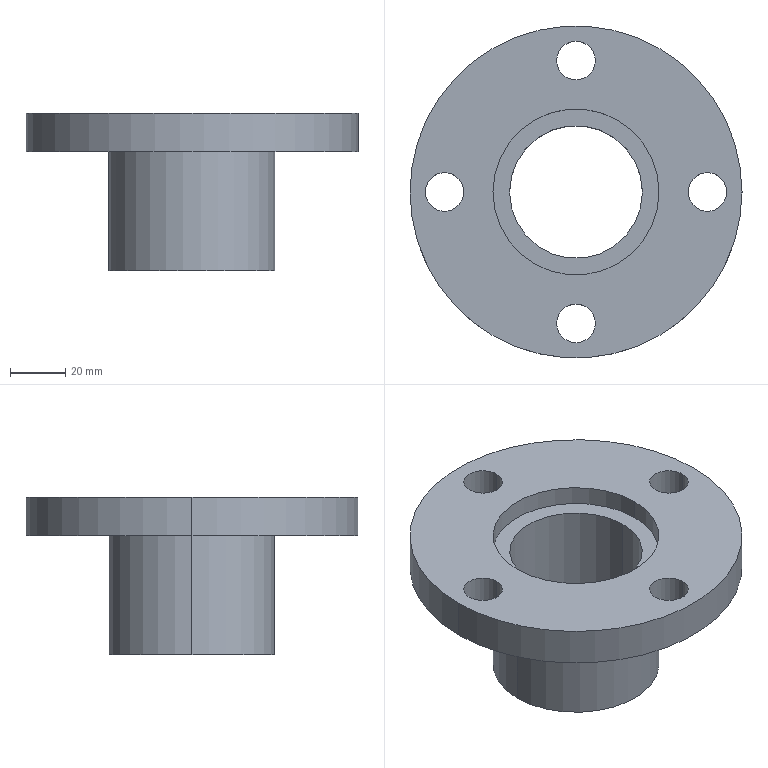Part | SolidWorks | features ExtruThin 1, HoleWzd 1, ICE 1 | 2 solids | 20 faces | box 120 x 120 x 57 mm | volume 161025 mm3 | cylinder 16 | plane 4 | commonest cylinder face diameters 14 x8 60 x4 48 x2 120 x2
STEP:
#1=CARTESIAN_POINT('',(-24.,0.,50.));
#2=VERTEX_POINT('',#1);
#3=CARTESIAN_POINT('',(24.,0.,50.));
#4=VERTEX_POINT('',#3);
#5=CARTESIAN_POINT('',(0.,0.,50.));
#6=DIRECTION('',(0.,0.,1.));
#7=DIRECTION('',(1.,0.,0.));
#8=AXIS2_PLACEMENT_3D('',#5,#6,#7);
#9=CIRCLE('',#8,24.);
#10=EDGE_CURVE('',#2,#4,#9,.T.);
#11=ORIENTED_EDGE('',*,*,#10,.T.);
#12=CARTESIAN_POINT('',(24.,0.,0.));
#13=VERTEX_POINT('',#12);
#14=CARTESIAN_POINT('',(24.,0.,50.));
#15=DIRECTION('',(0.,0.,-1.));
#16=VECTOR('',#15,1000.);
#17=LINE('',#14,#16);
#18=EDGE_CURVE('',#4,#13,#17,.T.);
#19=ORIENTED_EDGE('',*,*,#18,.T.);
#20=CARTESIAN_POINT('',(-24.,0.,0.));
#21=VERTEX_POINT('',#20);
#22=CARTESIAN_POINT('',(0.,0.,0.));
#23=DIRECTION('',(0.,0.,1.));
#24=DIRECTION('',(1.,0.,0.));
#25=AXIS2_PLACEMENT_3D('',#22,#23,#24);
#26=CIRCLE('',#25,24.);
#27=EDGE_CURVE('',#21,#13,#26,.T.);
#28=ORIENTED_EDGE('',*,*,#27,.F.);
#29=CARTESIAN_POINT('',(-24.,0.,50.));
#30=DIRECTION('',(0.,0.,-1.));
#31=VECTOR('',#30,1000.);
#32=LINE('',#29,#31);
#33=EDGE_CURVE('',#2,#21,#32,.T.);
#34=ORIENTED_EDGE('',*,*,#33,.F.);
#35=EDGE_LOOP('',(#11,#19,#28,#34));
#36=FACE_OUTER_BOUND('',#35,.T.);
#37=CARTESIAN_POINT('',(0.,0.,50.));
#38=DIRECTION('',(0.,0.,-1.));
#39=DIRECTION('',(-1.,0.,0.));
#40=AXIS2_PLACEMENT_3D('',#37,#38,#39);
#41=CYLINDRICAL_SURFACE('',#40,24.);
#42=ADVANCED_FACE('',(#36),#41,.F.);
#43=CARTESIAN_POINT('',(30.,0.,50.));
#44=VERTEX_POINT('',#43);
#45=CARTESIAN_POINT('',(-30.,0.,50.));
#46=VERTEX_POINT('',#45);
#47=CARTESIAN_POINT('',(0.,0.,50.));
#48=DIRECTION('',(0.,0.,1.));
#49=DIRECTION('',(1.,0.,0.));
#50=AXIS2_PLACEMENT_3D('',#47,#48,#49);
#51=CIRCLE('',#50,30.);
#52=EDGE_CURVE('',#44,#46,#51,.T.);
#53=ORIENTED_EDGE('',*,*,#52,.F.);
#54=CARTESIAN_POINT('',(30.,0.,0.));
#55=VERTEX_POINT('',#54);
#56=CARTESIAN_POINT('',(30.,0.,50.));
#57=DIRECTION('',(0.,0.,-1.));
#58=VECTOR('',#57,1000.);
#59=LINE('',#56,#58);
#60=EDGE_CURVE('',#44,#55,#59,.T.);
#61=ORIENTED_EDGE('',*,*,#60,.T.);
#62=CARTESIAN_POINT('',(-30.,0.,0.));
#63=VERTEX_POINT('',#62);
#64=CARTESIAN_POINT('',(0.,0.,0.));
#65=DIRECTION('',(0.,0.,1.));
#66=DIRECTION('',(1.,0.,0.));
#67=AXIS2_PLACEMENT_3D('',#64,#65,#66);
#68=CIRCLE('',#67,30.);
#69=EDGE_CURVE('',#55,#63,#68,.T.);
#70=ORIENTED_EDGE('',*,*,#69,.T.);
#71=CARTESIAN_POINT('',(-30.,0.,50.));
#72=DIRECTION('',(0.,0.,-1.));
#73=VECTOR('',#72,1000.);
#74=LINE('',#71,#73);
#75=EDGE_CURVE('',#46,#63,#74,.T.);
#76=ORIENTED_EDGE('',*,*,#75,.F.);
#77=EDGE_LOOP('',(#53,#61,#70,#76));
#78=FACE_OUTER_BOUND('',#77,.T.);
#79=CARTESIAN_POINT('',(0.,0.,50.));
#80=DIRECTION('',(0.,0.,-1.));
#81=DIRECTION('',(-1.,0.,0.));
#82=AXIS2_PLACEMENT_3D('',#79,#80,#81);
#83=CYLINDRICAL_SURFACE('',#82,30.);
#84=ADVANCED_FACE('',(#78),#83,.T.);
#85=CARTESIAN_POINT('',(0.,0.,50.));
#86=DIRECTION('',(0.,0.,1.));
#87=DIRECTION('',(1.,0.,0.));
#88=AXIS2_PLACEMENT_3D('',#85,#86,#87);
#89=CIRCLE('',#88,30.);
#90=EDGE_CURVE('',#46,#44,#89,.T.);
#91=ORIENTED_EDGE('',*,*,#90,.T.);
#92=ORIENTED_EDGE('',*,*,#52,.T.);
#93=EDGE_LOOP('',(#91,#92));
#94=FACE_OUTER_BOUND('',#93,.T.);
#95=ORIENTED_EDGE('',*,*,#10,.F.);
#96=CARTESIAN_POINT('',(0.,0.,50.));
#97=DIRECTION('',(0.,0.,1.));
#98=DIRECTION('',(1.,0.,0.));
#99=AXIS2_PLACEMENT_3D('',#96,#97,#98);
#100=CIRCLE('',#99,24.);
#101=EDGE_CURVE('',#4,#2,#100,.T.);
#102=ORIENTED_EDGE('',*,*,#101,.F.);
#103=EDGE_LOOP('',(#95,#102));
#104=FACE_BOUND('',#103,.T.);
#105=CARTESIAN_POINT('',(0.,0.,50.));
#106=DIRECTION('',(0.,0.,1.));
#107=DIRECTION('',(1.,0.,0.));
#108=AXIS2_PLACEMENT_3D('',#105,#106,#107);
#109=PLANE('',#108);
#110=ADVANCED_FACE('',(#94,#104),#109,.T.);
#111=CARTESIAN_POINT('',(0.,0.,0.));
#112=DIRECTION('',(0.,0.,1.));
#113=DIRECTION('',(1.,0.,0.));
#114=AXIS2_PLACEMENT_3D('',#111,#112,#113);
#115=CIRCLE('',#114,30.);
#116=EDGE_CURVE('',#63,#55,#115,.T.);
#117=ORIENTED_EDGE('',*,*,#116,.F.);
#118=ORIENTED_EDGE('',*,*,#69,.F.);
#119=EDGE_LOOP('',(#117,#118));
#120=FACE_OUTER_BOUND('',#119,.T.);
#121=ORIENTED_EDGE('',*,*,#27,.T.);
#122=CARTESIAN_POINT('',(0.,0.,0.));
#123=DIRECTION('',(0.,0.,1.));
#124=DIRECTION('',(1.,0.,0.));
#125=AXIS2_PLACEMENT_3D('',#122,#123,#124);
#126=CIRCLE('',#125,24.);
#127=EDGE_CURVE('',#13,#21,#126,.T.);
#128=ORIENTED_EDGE('',*,*,#127,.T.);
#129=EDGE_LOOP('',(#121,#128));
#130=FACE_BOUND('',#129,.T.);
#131=CARTESIAN_POINT('',(0.,0.,0.));
#132=DIRECTION('',(0.,0.,1.));
#133=DIRECTION('',(1.,0.,0.));
#134=AXIS2_PLACEMENT_3D('',#131,#132,#133);
#135=PLANE('',#134);
#136=ADVANCED_FACE('',(#120,#130),#135,.F.);
#137=ORIENTED_EDGE('',*,*,#60,.F.);
#138=ORIENTED_EDGE('',*,*,#90,.F.);
#139=ORIENTED_EDGE('',*,*,#75,.T.);
#140=ORIENTED_EDGE('',*,*,#116,.T.);
#141=EDGE_LOOP('',(#137,#138,#139,#140));
#142=FACE_OUTER_BOUND('',#141,.T.);
#143=CARTESIAN_POINT('',(0.,0.,50.));
#144=DIRECTION('',(0.,0.,-1.));
#145=DIRECTION('',(-1.,0.,0.));
#146=AXIS2_PLACEMENT_3D('',#143,#144,#145);
#147=CYLINDRICAL_SURFACE('',#146,30.);
#148=ADVANCED_FACE('',(#142),#147,.T.);
#149=ORIENTED_EDGE('',*,*,#18,.F.);
#150=ORIENTED_EDGE('',*,*,#101,.T.);
#151=ORIENTED_EDGE('',*,*,#33,.T.);
#152=ORIENTED_EDGE('',*,*,#127,.F.);
#153=EDGE_LOOP('',(#149,#150,#151,#152));
#154=FACE_OUTER_BOUND('',#153,.T.);
#155=CARTESIAN_POINT('',(0.,0.,50.));
#156=DIRECTION('',(0.,0.,-1.));
#157=DIRECTION('',(-1.,0.,0.));
#158=AXIS2_PLACEMENT_3D('',#155,#156,#157);
#159=CYLINDRICAL_SURFACE('',#158,24.);
#160=ADVANCED_FACE('',(#154),#159,.F.);
#161=CLOSED_SHELL('',(#42,#84,#110,#136,#148,#160));
#162=MANIFOLD_SOLID_BREP('',#161);
#163=CARTESIAN_POINT('',(-7.,47.5,43.));
#164=VERTEX_POINT('',#163);
#165=CARTESIAN_POINT('',(7.,47.5,43.));
#166=VERTEX_POINT('',#165);
#167=CARTESIAN_POINT('',(0.,47.5,43.));
#168=DIRECTION('',(0.,0.,1.));
#169=DIRECTION('',(1.,0.,0.));
#170=AXIS2_PLACEMENT_3D('',#167,#168,#169);
#171=CIRCLE('',#170,7.);
#172=EDGE_CURVE('',#164,#166,#171,.T.);
#173=ORIENTED_EDGE('',*,*,#172,.F.);
#174=CARTESIAN_POINT('',(-7.,47.5,57.));
#175=VERTEX_POINT('',#174);
#176=CARTESIAN_POINT('',(-7.,47.5,57.));
#177=DIRECTION('',(0.,0.,1.));
#178=VECTOR('',#177,1000.);
#179=LINE('',#176,#178);
#180=EDGE_CURVE('',#164,#175,#179,.T.);
#181=ORIENTED_EDGE('',*,*,#180,.T.);
#182=CARTESIAN_POINT('',(7.,47.5,57.));
#183=VERTEX_POINT('',#182);
#184=CARTESIAN_POINT('',(0.,47.5,57.));
#185=DIRECTION('',(0.,0.,1.));
#186=DIRECTION('',(1.,0.,0.));
#187=AXIS2_PLACEMENT_3D('',#184,#185,#186);
#188=CIRCLE('',#187,7.);
#189=EDGE_CURVE('',#175,#183,#188,.T.);
#190=ORIENTED_EDGE('',*,*,#189,.T.);
#191=CARTESIAN_POINT('',(7.,47.5,57.));
#192=DIRECTION('',(0.,0.,1.));
#193=VECTOR('',#192,1000.);
#194=LINE('',#191,#193);
#195=EDGE_CURVE('',#166,#183,#194,.T.);
#196=ORIENTED_EDGE('',*,*,#195,.F.);
#197=EDGE_LOOP('',(#173,#181,#190,#196));
#198=FACE_OUTER_BOUND('',#197,.T.);
#199=CARTESIAN_POINT('',(0.,47.5,57.));
#200=DIRECTION('',(0.,0.,1.));
#201=DIRECTION('',(1.,0.,0.));
#202=AXIS2_PLACEMENT_3D('',#199,#200,#201);
#203=CYLINDRICAL_SURFACE('',#202,7.);
#204=ADVANCED_FACE('',(#198),#203,.F.);
#205=CARTESIAN_POINT('',(-54.5,0.,43.));
#206=VERTEX_POINT('',#205);
#207=CARTESIAN_POINT('',(-40.5,0.,43.));
#208=VERTEX_POINT('',#207);
#209=CARTESIAN_POINT('',(-47.5,0.,43.));
#210=DIRECTION('',(0.,0.,1.));
#211=DIRECTION('',(1.,0.,0.));
#212=AXIS2_PLACEMENT_3D('',#209,#210,#211);
#213=CIRCLE('',#212,7.);
#214=EDGE_CURVE('',#206,#208,#213,.T.);
#215=ORIENTED_EDGE('',*,*,#214,.F.);
#216=CARTESIAN_POINT('',(-54.5,0.,57.));
#217=VERTEX_POINT('',#216);
#218=CARTESIAN_POINT('',(-54.5,0.,57.));
#219=DIRECTION('',(0.,0.,1.));
#220=VECTOR('',#219,1000.);
#221=LINE('',#218,#220);
#222=EDGE_CURVE('',#206,#217,#221,.T.);
#223=ORIENTED_EDGE('',*,*,#222,.T.);
#224=CARTESIAN_POINT('',(-40.5,0.,57.));
#225=VERTEX_POINT('',#224);
#226=CARTESIAN_POINT('',(-47.5,0.,57.));
#227=DIRECTION('',(0.,0.,1.));
#228=DIRECTION('',(1.,0.,0.));
#229=AXIS2_PLACEMENT_3D('',#226,#227,#228);
#230=CIRCLE('',#229,7.);
#231=EDGE_CURVE('',#217,#225,#230,.T.);
#232=ORIENTED_EDGE('',*,*,#231,.T.);
#233=CARTESIAN_POINT('',(-40.5,0.,57.));
#234=DIRECTION('',(0.,0.,1.));
#235=VECTOR('',#234,1000.);
#236=LINE('',#233,#235);
#237=EDGE_CURVE('',#208,#225,#236,.T.);
#238=ORIENTED_EDGE('',*,*,#237,.F.);
#239=EDGE_LOOP('',(#215,#223,#232,#238));
#240=FACE_OUTER_BOUND('',#239,.T.);
#241=CARTESIAN_POINT('',(-47.5,0.,57.));
#242=DIRECTION('',(0.,0.,1.));
#243=DIRECTION('',(1.,0.,0.));
#244=AXIS2_PLACEMENT_3D('',#241,#242,#243);
#245=CYLINDRICAL_SURFACE('',#244,7.);
#246=ADVANCED_FACE('',(#240),#245,.F.);
#247=CARTESIAN_POINT('',(40.5,0.,43.));
#248=VERTEX_POINT('',#247);
#249=CARTESIAN_POINT('',(54.5,0.,43.));
#250=VERTEX_POINT('',#249);
#251=CARTESIAN_POINT('',(47.5,0.,43.));
#252=DIRECTION('',(0.,0.,1.));
#253=DIRECTION('',(1.,0.,0.));
#254=AXIS2_PLACEMENT_3D('',#251,#252,#253);
#255=CIRCLE('',#254,7.);
#256=EDGE_CURVE('',#248,#250,#255,.T.);
#257=ORIENTED_EDGE('',*,*,#256,.F.);
#258=CARTESIAN_POINT('',(40.5,0.,57.));
#259=VERTEX_POINT('',#258);
#260=CARTESIAN_POINT('',(40.5,0.,57.));
#261=DIRECTION('',(0.,0.,1.));
#262=VECTOR('',#261,1000.);
#263=LINE('',#260,#262);
#264=EDGE_CURVE('',#248,#259,#263,.T.);
#265=ORIENTED_EDGE('',*,*,#264,.T.);
#266=CARTESIAN_POINT('',(54.5,0.,57.));
#267=VERTEX_POINT('',#266);
#268=CARTESIAN_POINT('',(47.5,0.,57.));
#269=DIRECTION('',(0.,0.,1.));
#270=DIRECTION('',(1.,0.,0.));
#271=AXIS2_PLACEMENT_3D('',#268,#269,#270);
#272=CIRCLE('',#271,7.);
#273=EDGE_CURVE('',#259,#267,#272,.T.);
#274=ORIENTED_EDGE('',*,*,#273,.T.);
#275=CARTESIAN_POINT('',(54.5,0.,57.));
#276=DIRECTION('',(0.,0.,1.));
#277=VECTOR('',#276,1000.);
#278=LINE('',#275,#277);
#279=EDGE_CURVE('',#250,#267,#278,.T.);
#280=ORIENTED_EDGE('',*,*,#279,.F.);
#281=EDGE_LOOP('',(#257,#265,#274,#280));
#282=FACE_OUTER_BOUND('',#281,.T.);
#283=CARTESIAN_POINT('',(47.5,0.,57.));
#284=DIRECTION('',(0.,0.,1.));
#285=DIRECTION('',(1.,0.,0.));
#286=AXIS2_PLACEMENT_3D('',#283,#284,#285);
#287=CYLINDRICAL_SURFACE('',#286,7.);
#288=ADVANCED_FACE('',(#282),#287,.F.);
#289=CARTESIAN_POINT('',(-7.,-47.5,43.));
#290=VERTEX_POINT('',#289);
#291=CARTESIAN_POINT('',(7.,-47.5,43.));
#292=VERTEX_POINT('',#291);
#293=CARTESIAN_POINT('',(0.,-47.5,43.));
#294=DIRECTION('',(0.,0.,1.));
#295=DIRECTION('',(1.,0.,0.));
#296=AXIS2_PLACEMENT_3D('',#293,#294,#295);
#297=CIRCLE('',#296,7.);
#298=EDGE_CURVE('',#290,#292,#297,.T.);
#299=ORIENTED_EDGE('',*,*,#298,.F.);
#300=CARTESIAN_POINT('',(-7.,-47.5,57.));
#301=VERTEX_POINT('',#300);
#302=CARTESIAN_POINT('',(-7.,-47.5,57.));
#303=DIRECTION('',(0.,0.,1.));
#304=VECTOR('',#303,1000.);
#305=LINE('',#302,#304);
#306=EDGE_CURVE('',#290,#301,#305,.T.);
#307=ORIENTED_EDGE('',*,*,#306,.T.);
#308=CARTESIAN_POINT('',(7.,-47.5,57.));
#309=VERTEX_POINT('',#308);
#310=CARTESIAN_POINT('',(0.,-47.5,57.));
#311=DIRECTION('',(0.,0.,1.));
#312=DIRECTION('',(1.,0.,0.));
#313=AXIS2_PLACEMENT_3D('',#310,#311,#312);
#314=CIRCLE('',#313,7.);
#315=EDGE_CURVE('',#301,#309,#314,.T.);
#316=ORIENTED_EDGE('',*,*,#315,.T.);
#317=CARTESIAN_POINT('',(7.,-47.5,57.));
#318=DIRECTION('',(0.,0.,1.));
#319=VECTOR('',#318,1000.);
#320=LINE('',#317,#319);
#321=EDGE_CURVE('',#292,#309,#320,.T.);
#322=ORIENTED_EDGE('',*,*,#321,.F.);
#323=EDGE_LOOP('',(#299,#307,#316,#322));
#324=FACE_OUTER_BOUND('',#323,.T.);
#325=CARTESIAN_POINT('',(0.,-47.5,57.));
#326=DIRECTION('',(0.,0.,1.));
#327=DIRECTION('',(1.,0.,0.));
#328=AXIS2_PLACEMENT_3D('',#325,#326,#327);
#329=CYLINDRICAL_SURFACE('',#328,7.);
#330=ADVANCED_FACE('',(#324),#329,.F.);
#331=CARTESIAN_POINT('',(-30.,0.,57.));
#332=VERTEX_POINT('',#331);
#333=CARTESIAN_POINT('',(30.,0.,57.));
#334=VERTEX_POINT('',#333);
#335=CARTESIAN_POINT('',(0.,0.,57.));
#336=DIRECTION('',(0.,0.,1.));
#337=DIRECTION('',(1.,0.,0.));
#338=AXIS2_PLACEMENT_3D('',#335,#336,#337);
#339=CIRCLE('',#338,30.);
#340=EDGE_CURVE('',#332,#334,#339,.T.);
#341=ORIENTED_EDGE('',*,*,#340,.T.);
#342=CARTESIAN_POINT('',(30.,0.,43.));
#343=VERTEX_POINT('',#342);
#344=CARTESIAN_POINT('',(30.,0.,57.));
#345=DIRECTION('',(0.,0.,-1.));
#346=VECTOR('',#345,1000.);
#347=LINE('',#344,#346);
#348=EDGE_CURVE('',#334,#343,#347,.T.);
#349=ORIENTED_EDGE('',*,*,#348,.T.);
#350=CARTESIAN_POINT('',(-30.,0.,43.));
#351=VERTEX_POINT('',#350);
#352=CARTESIAN_POINT('',(0.,0.,43.));
#353=DIRECTION('',(0.,0.,1.));
#354=DIRECTION('',(1.,0.,0.));
#355=AXIS2_PLACEMENT_3D('',#352,#353,#354);
#356=CIRCLE('',#355,30.);
#357=EDGE_CURVE('',#351,#343,#356,.T.);
#358=ORIENTED_EDGE('',*,*,#357,.F.);
#359=CARTESIAN_POINT('',(-30.,0.,57.));
#360=DIRECTION('',(0.,0.,-1.));
#361=VECTOR('',#360,1000.);
#362=LINE('',#359,#361);
#363=EDGE_CURVE('',#332,#351,#362,.T.);
#364=ORIENTED_EDGE('',*,*,#363,.F.);
#365=EDGE_LOOP('',(#341,#349,#358,#364));
#366=FACE_OUTER_BOUND('',#365,.T.);
#367=CARTESIAN_POINT('',(0.,0.,57.));
#368=DIRECTION('',(0.,0.,-1.));
#369=DIRECTION('',(-1.,0.,0.));
#370=AXIS2_PLACEMENT_3D('',#367,#368,#369);
#371=CYLINDRICAL_SURFACE('',#370,30.);
#372=ADVANCED_FACE('',(#366),#371,.F.);
#373=CARTESIAN_POINT('',(60.,0.,57.));
#374=VERTEX_POINT('',#373);
#375=CARTESIAN_POINT('',(-60.,0.,57.));
#376=VERTEX_POINT('',#375);
#377=CARTESIAN_POINT('',(0.,0.,57.));
#378=DIRECTION('',(0.,0.,1.));
#379=DIRECTION('',(1.,0.,0.));
#380=AXIS2_PLACEMENT_3D('',#377,#378,#379);
#381=CIRCLE('',#380,60.);
#382=EDGE_CURVE('',#374,#376,#381,.T.);
#383=ORIENTED_EDGE('',*,*,#382,.F.);
#384=CARTESIAN_POINT('',(60.,0.,43.));
#385=VERTEX_POINT('',#384);
#386=CARTESIAN_POINT('',(60.,0.,57.));
#387=DIRECTION('',(0.,0.,-1.));
#388=VECTOR('',#387,1000.);
#389=LINE('',#386,#388);
#390=EDGE_CURVE('',#374,#385,#389,.T.);
#391=ORIENTED_EDGE('',*,*,#390,.T.);
#392=CARTESIAN_POINT('',(-60.,0.,43.));
#393=VERTEX_POINT('',#392);
#394=CARTESIAN_POINT('',(0.,0.,43.));
#395=DIRECTION('',(0.,0.,1.));
#396=DIRECTION('',(1.,0.,0.));
#397=AXIS2_PLACEMENT_3D('',#394,#395,#396);
#398=CIRCLE('',#397,60.);
#399=EDGE_CURVE('',#385,#393,#398,.T.);
#400=ORIENTED_EDGE('',*,*,#399,.T.);
#401=CARTESIAN_POINT('',(-60.,0.,57.));
#402=DIRECTION('',(0.,0.,-1.));
#403=VECTOR('',#402,1000.);
#404=LINE('',#401,#403);
#405=EDGE_CURVE('',#376,#393,#404,.T.);
#406=ORIENTED_EDGE('',*,*,#405,.F.);
#407=EDGE_LOOP('',(#383,#391,#400,#406));
#408=FACE_OUTER_BOUND('',#407,.T.);
#409=CARTESIAN_POINT('',(0.,0.,57.));
#410=DIRECTION('',(0.,0.,-1.));
#411=DIRECTION('',(-1.,0.,0.));
#412=AXIS2_PLACEMENT_3D('',#409,#410,#411);
#413=CYLINDRICAL_SURFACE('',#412,60.);
#414=ADVANCED_FACE('',(#408),#413,.T.);
#415=CARTESIAN_POINT('',(0.,47.5,57.));
#416=DIRECTION('',(0.,0.,1.));
#417=DIRECTION('',(1.,0.,0.));
#418=AXIS2_PLACEMENT_3D('',#415,#416,#417);
#419=CIRCLE('',#418,7.);
#420=EDGE_CURVE('',#183,#175,#419,.T.);
#421=ORIENTED_EDGE('',*,*,#420,.F.);
#422=ORIENTED_EDGE('',*,*,#189,.F.);
#423=EDGE_LOOP('',(#421,#422));
#424=FACE_BOUND('',#423,.T.);
#425=CARTESIAN_POINT('',(-47.5,0.,57.));
#426=DIRECTION('',(0.,0.,1.));
#427=DIRECTION('',(1.,0.,0.));
#428=AXIS2_PLACEMENT_3D('',#425,#426,#427);
#429=CIRCLE('',#428,7.);
#430=EDGE_CURVE('',#225,#217,#429,.T.);
#431=ORIENTED_EDGE('',*,*,#430,.F.);
#432=ORIENTED_EDGE('',*,*,#231,.F.);
#433=EDGE_LOOP('',(#431,#432));
#434=FACE_BOUND('',#433,.T.);
#435=CARTESIAN_POINT('',(47.5,0.,57.));
#436=DIRECTION('',(0.,0.,1.));
#437=DIRECTION('',(1.,0.,0.));
#438=AXIS2_PLACEMENT_3D('',#435,#436,#437);
#439=CIRCLE('',#438,7.);
#440=EDGE_CURVE('',#267,#259,#439,.T.);
#441=ORIENTED_EDGE('',*,*,#440,.F.);
#442=ORIENTED_EDGE('',*,*,#273,.F.);
#443=EDGE_LOOP('',(#441,#442));
#444=FACE_BOUND('',#443,.T.);
#445=CARTESIAN_POINT('',(0.,-47.5,57.));
#446=DIRECTION('',(0.,0.,1.));
#447=DIRECTION('',(1.,0.,0.));
#448=AXIS2_PLACEMENT_3D('',#445,#446,#447);
#449=CIRCLE('',#448,7.);
#450=EDGE_CURVE('',#309,#301,#449,.T.);
#451=ORIENTED_EDGE('',*,*,#450,.F.);
#452=ORIENTED_EDGE('',*,*,#315,.F.);
#453=EDGE_LOOP('',(#451,#452));
#454=FACE_BOUND('',#453,.T.);
#455=CARTESIAN_POINT('',(0.,0.,57.));
#456=DIRECTION('',(0.,0.,1.));
#457=DIRECTION('',(1.,0.,0.));
#458=AXIS2_PLACEMENT_3D('',#455,#456,#457);
#459=CIRCLE('',#458,60.);
#460=EDGE_CURVE('',#376,#374,#459,.T.);
#461=ORIENTED_EDGE('',*,*,#460,.T.);
#462=ORIENTED_EDGE('',*,*,#382,.T.);
#463=EDGE_LOOP('',(#461,#462));
#464=FACE_OUTER_BOUND('',#463,.T.);
#465=ORIENTED_EDGE('',*,*,#340,.F.);
#466=CARTESIAN_POINT('',(0.,0.,57.));
#467=DIRECTION('',(0.,0.,1.));
#468=DIRECTION('',(1.,0.,0.));
#469=AXIS2_PLACEMENT_3D('',#466,#467,#468);
#470=CIRCLE('',#469,30.);
#471=EDGE_CURVE('',#334,#332,#470,.T.);
#472=ORIENTED_EDGE('',*,*,#471,.F.);
#473=EDGE_LOOP('',(#465,#472));
#474=FACE_BOUND('',#473,.T.);
#475=CARTESIAN_POINT('',(0.,0.,57.));
#476=DIRECTION('',(0.,0.,1.));
#477=DIRECTION('',(1.,0.,0.));
#478=AXIS2_PLACEMENT_3D('',#475,#476,#477);
#479=PLANE('',#478);
#480=ADVANCED_FACE('',(#424,#434,#444,#454,#464,#474),#479,.T.);
#481=CARTESIAN_POINT('',(0.,47.5,43.));
#482=DIRECTION('',(0.,0.,1.));
#483=DIRECTION('',(1.,0.,0.));
#484=AXIS2_PLACEMENT_3D('',#481,#482,#483);
#485=CIRCLE('',#484,7.);
#486=EDGE_CURVE('',#166,#164,#485,.T.);
#487=ORIENTED_EDGE('',*,*,#486,.T.);
#488=ORIENTED_EDGE('',*,*,#172,.T.);
#489=EDGE_LOOP('',(#487,#488));
#490=FACE_BOUND('',#489,.T.);
#491=CARTESIAN_POINT('',(-47.5,0.,43.));
#492=DIRECTION('',(0.,0.,1.));
#493=DIRECTION('',(1.,0.,0.));
#494=AXIS2_PLACEMENT_3D('',#491,#492,#493);
#495=CIRCLE('',#494,7.);
#496=EDGE_CURVE('',#208,#206,#495,.T.);
#497=ORIENTED_EDGE('',*,*,#496,.T.);
#498=ORIENTED_EDGE('',*,*,#214,.T.);
#499=EDGE_LOOP('',(#497,#498));
#500=FACE_BOUND('',#499,.T.);
#501=CARTESIAN_POINT('',(47.5,0.,43.));
#502=DIRECTION('',(0.,0.,1.));
#503=DIRECTION('',(1.,0.,0.));
#504=AXIS2_PLACEMENT_3D('',#501,#502,#503);
#505=CIRCLE('',#504,7.);
#506=EDGE_CURVE('',#250,#248,#505,.T.);
#507=ORIENTED_EDGE('',*,*,#506,.T.);
#508=ORIENTED_EDGE('',*,*,#256,.T.);
#509=EDGE_LOOP('',(#507,#508));
#510=FACE_BOUND('',#509,.T.);
#511=CARTESIAN_POINT('',(0.,-47.5,43.));
#512=DIRECTION('',(0.,0.,1.));
#513=DIRECTION('',(1.,0.,0.));
#514=AXIS2_PLACEMENT_3D('',#511,#512,#513);
#515=CIRCLE('',#514,7.);
#516=EDGE_CURVE('',#292,#290,#515,.T.);
#517=ORIENTED_EDGE('',*,*,#516,.T.);
#518=ORIENTED_EDGE('',*,*,#298,.T.);
#519=EDGE_LOOP('',(#517,#518));
#520=FACE_BOUND('',#519,.T.);
#521=CARTESIAN_POINT('',(0.,0.,43.));
#522=DIRECTION('',(0.,0.,1.));
#523=DIRECTION('',(1.,0.,0.));
#524=AXIS2_PLACEMENT_3D('',#521,#522,#523);
#525=CIRCLE('',#524,60.);
#526=EDGE_CURVE('',#393,#385,#525,.T.);
#527=ORIENTED_EDGE('',*,*,#526,.F.);
#528=ORIENTED_EDGE('',*,*,#399,.F.);
#529=EDGE_LOOP('',(#527,#528));
#530=FACE_OUTER_BOUND('',#529,.T.);
#531=ORIENTED_EDGE('',*,*,#357,.T.);
#532=CARTESIAN_POINT('',(0.,0.,43.));
#533=DIRECTION('',(0.,0.,1.));
#534=DIRECTION('',(1.,0.,0.));
#535=AXIS2_PLACEMENT_3D('',#532,#533,#534);
#536=CIRCLE('',#535,30.);
#537=EDGE_CURVE('',#343,#351,#536,.T.);
#538=ORIENTED_EDGE('',*,*,#537,.T.);
#539=EDGE_LOOP('',(#531,#538));
#540=FACE_BOUND('',#539,.T.);
#541=CARTESIAN_POINT('',(0.,0.,43.));
#542=DIRECTION('',(0.,0.,1.));
#543=DIRECTION('',(1.,0.,0.));
#544=AXIS2_PLACEMENT_3D('',#541,#542,#543);
#545=PLANE('',#544);
#546=ADVANCED_FACE('',(#490,#500,#510,#520,#530,#540),#545,.F.);
#547=ORIENTED_EDGE('',*,*,#390,.F.);
#548=ORIENTED_EDGE('',*,*,#460,.F.);
#549=ORIENTED_EDGE('',*,*,#405,.T.);
#550=ORIENTED_EDGE('',*,*,#526,.T.);
#551=EDGE_LOOP('',(#547,#548,#549,#550));
#552=FACE_OUTER_BOUND('',#551,.T.);
#553=CARTESIAN_POINT('',(0.,0.,57.));
#554=DIRECTION('',(0.,0.,-1.));
#555=DIRECTION('',(-1.,0.,0.));
#556=AXIS2_PLACEMENT_3D('',#553,#554,#555);
#557=CYLINDRICAL_SURFACE('',#556,60.);
#558=ADVANCED_FACE('',(#552),#557,.T.);
#559=ORIENTED_EDGE('',*,*,#348,.F.);
#560=ORIENTED_EDGE('',*,*,#471,.T.);
#561=ORIENTED_EDGE('',*,*,#363,.T.);
#562=ORIENTED_EDGE('',*,*,#537,.F.);
#563=EDGE_LOOP('',(#559,#560,#561,#562));
#564=FACE_OUTER_BOUND('',#563,.T.);
#565=CARTESIAN_POINT('',(0.,0.,57.));
#566=DIRECTION('',(0.,0.,-1.));
#567=DIRECTION('',(-1.,0.,0.));
#568=AXIS2_PLACEMENT_3D('',#565,#566,#567);
#569=CYLINDRICAL_SURFACE('',#568,30.);
#570=ADVANCED_FACE('',(#564),#569,.F.);
#571=ORIENTED_EDGE('',*,*,#306,.F.);
#572=ORIENTED_EDGE('',*,*,#516,.F.);
#573=ORIENTED_EDGE('',*,*,#321,.T.);
#574=ORIENTED_EDGE('',*,*,#450,.T.);
#575=EDGE_LOOP('',(#571,#572,#573,#574));
#576=FACE_OUTER_BOUND('',#575,.T.);
#577=CARTESIAN_POINT('',(0.,-47.5,57.));
#578=DIRECTION('',(0.,0.,1.));
#579=DIRECTION('',(1.,0.,0.));
#580=AXIS2_PLACEMENT_3D('',#577,#578,#579);
#581=CYLINDRICAL_SURFACE('',#580,7.);
#582=ADVANCED_FACE('',(#576),#581,.F.);
#583=ORIENTED_EDGE('',*,*,#264,.F.);
#584=ORIENTED_EDGE('',*,*,#506,.F.);
#585=ORIENTED_EDGE('',*,*,#279,.T.);
#586=ORIENTED_EDGE('',*,*,#440,.T.);
#587=EDGE_LOOP('',(#583,#584,#585,#586));
#588=FACE_OUTER_BOUND('',#587,.T.);
#589=CARTESIAN_POINT('',(47.5,0.,57.));
#590=DIRECTION('',(0.,0.,1.));
#591=DIRECTION('',(1.,0.,0.));
#592=AXIS2_PLACEMENT_3D('',#589,#590,#591);
#593=CYLINDRICAL_SURFACE('',#592,7.);
#594=ADVANCED_FACE('',(#588),#593,.F.);
#595=ORIENTED_EDGE('',*,*,#222,.F.);
#596=ORIENTED_EDGE('',*,*,#496,.F.);
#597=ORIENTED_EDGE('',*,*,#237,.T.);
#598=ORIENTED_EDGE('',*,*,#430,.T.);
#599=EDGE_LOOP('',(#595,#596,#597,#598));
#600=FACE_OUTER_BOUND('',#599,.T.);
#601=CARTESIAN_POINT('',(-47.5,0.,57.));
#602=DIRECTION('',(0.,0.,1.));
#603=DIRECTION('',(1.,0.,0.));
#604=AXIS2_PLACEMENT_3D('',#601,#602,#603);
#605=CYLINDRICAL_SURFACE('',#604,7.);
#606=ADVANCED_FACE('',(#600),#605,.F.);
#607=ORIENTED_EDGE('',*,*,#180,.F.);
#608=ORIENTED_EDGE('',*,*,#486,.F.);
#609=ORIENTED_EDGE('',*,*,#195,.T.);
#610=ORIENTED_EDGE('',*,*,#420,.T.);
#611=EDGE_LOOP('',(#607,#608,#609,#610));
#612=FACE_OUTER_BOUND('',#611,.T.);
#613=CARTESIAN_POINT('',(0.,47.5,57.));
#614=DIRECTION('',(0.,0.,1.));
#615=DIRECTION('',(1.,0.,0.));
#616=AXIS2_PLACEMENT_3D('',#613,#614,#615);
#617=CYLINDRICAL_SURFACE('',#616,7.);
#618=ADVANCED_FACE('',(#612),#617,.F.);
#619=CLOSED_SHELL('',(#204,#246,#288,#330,#372,#414,#480,#546,#558,#570,#582,#594,#606,#618));
#620=MANIFOLD_SOLID_BREP('',#619);
#621=CARTESIAN_POINT('',(0.,0.,0.));
#622=DIRECTION('',(0.,0.,1.));
#623=DIRECTION('',(1.,0.,0.));
#624=AXIS2_PLACEMENT_3D('',#621,#622,#623);
#625=(LENGTH_UNIT()NAMED_UNIT(*)SI_UNIT(.MILLI.,.METRE.));
#626=UNCERTAINTY_MEASURE_WITH_UNIT(LENGTH_MEASURE(0.00001),#625,'','');
#627=(NAMED_UNIT(*)PLANE_ANGLE_UNIT()SI_UNIT($,.RADIAN.));
#628=(NAMED_UNIT(*)SI_UNIT($,.STERADIAN.)SOLID_ANGLE_UNIT());
#629=(GEOMETRIC_REPRESENTATION_CONTEXT(3)GLOBAL_UNCERTAINTY_ASSIGNED_CONTEXT((#626))GLOBAL_UNIT_ASSIGNED_CONTEXT((#625,#627,#628))REPRESENTATION_CONTEXT('',''));
#630=ADVANCED_BREP_SHAPE_REPRESENTATION('',(#162,#620,#624),#629);